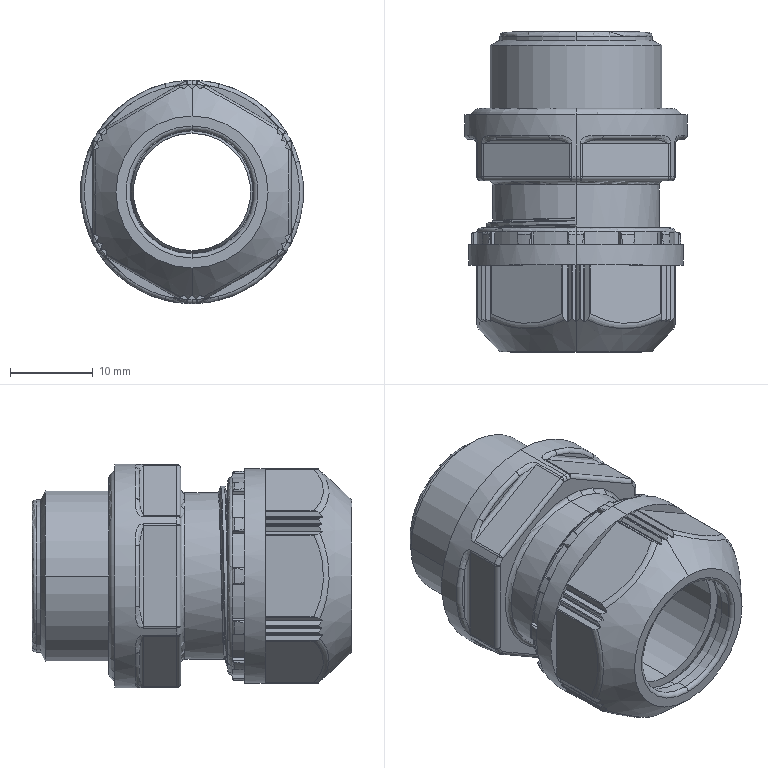Part | STEP file | G3L22N30-MM02TNNTNXH6-Part-2 | 1 solid | 445 faces | box 27 x 38.701 x 27 mm | volume 9074 mm3 | cylinder 153 | plane 116 | torus 68 | cone 48 | spline 48 | sphere 12 | commonest cylinder face diameters 0.2 x56 0.6 x32 1 x24 24 x12 20.2 x3 14.2 x2